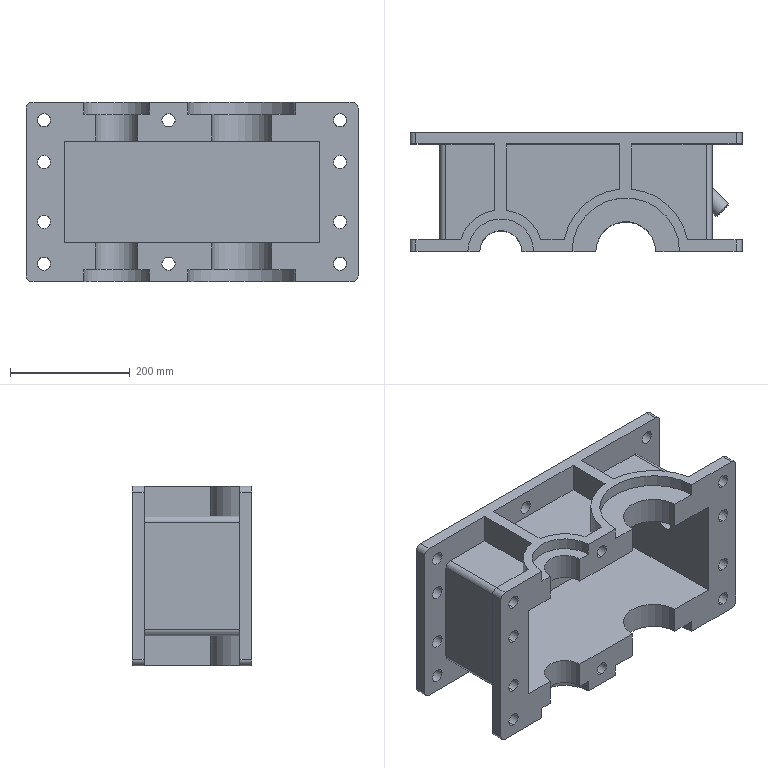Part | SolidWorks | features ICE 10, Chamfer 1, Extrusion 1, Fillet 1, MirrorPattern 1, Revolution 1, Shell 1 | 1 solid | 119 faces | box 555 x 200 x 300 mm | volume 8643514 mm3 | cylinder 72 | plane 45 | cone 2 | commonest cylinder face diameters 22 x40 20 x12 140 x4 210 x4 18 x2 30 x2